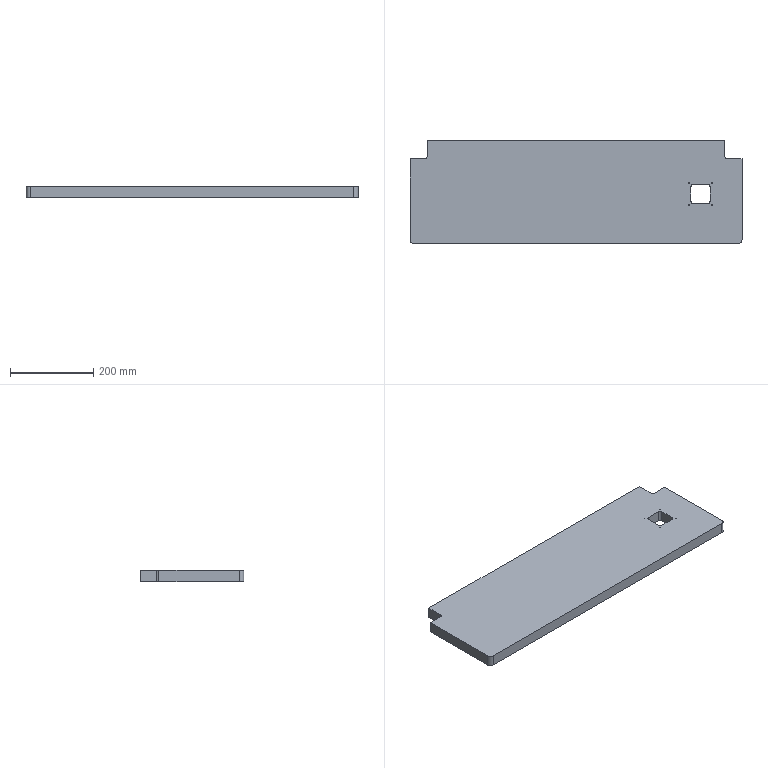Part | STEP file | Tabletop plate | 1 solid | 30 faces | box 800 x 250 x 27 mm | volume 5242609 mm3 | cylinder 16 | plane 14 | commonest cylinder face diameters 2 x8 10 x6 20 x2